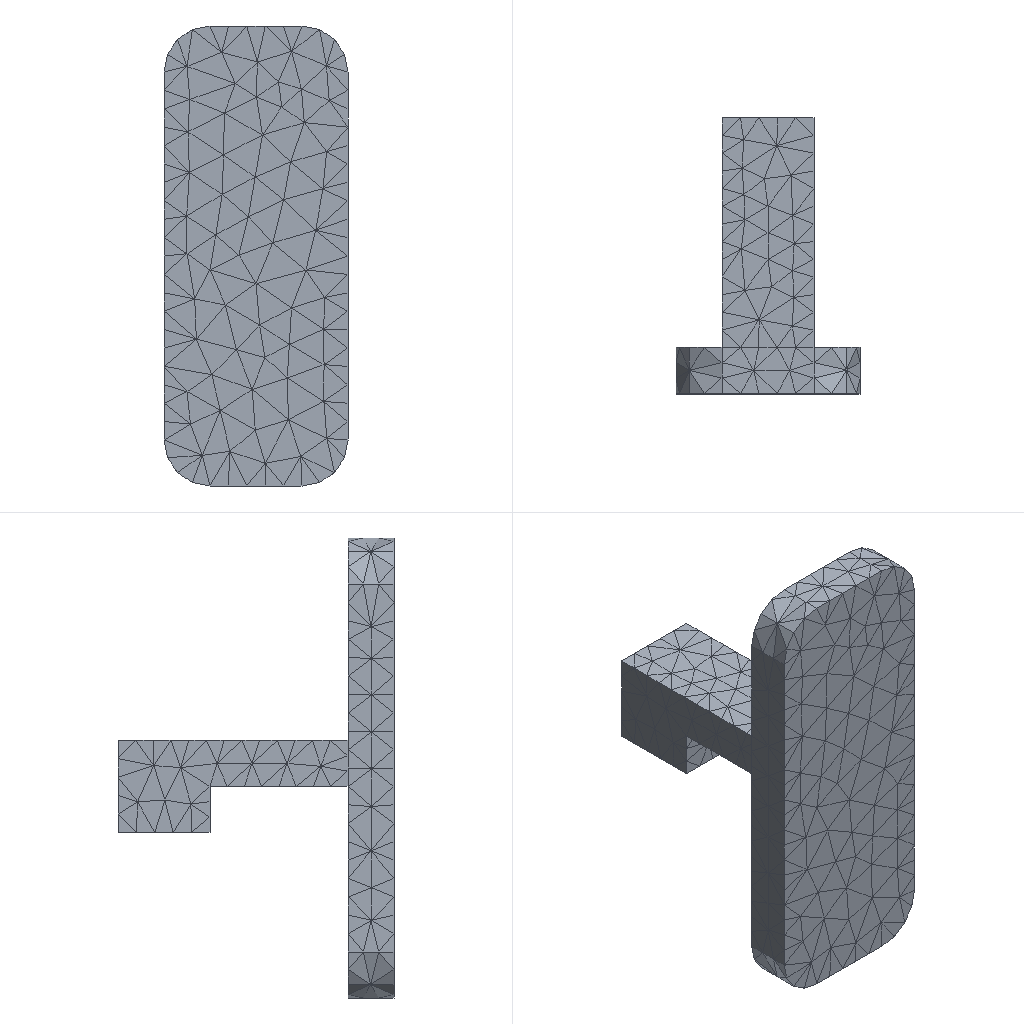Simulation study | ansys workbench
Ansys APDL input file, long lists of numbers shortened:
/batch
/config,noeldb,1     ! force off writing results to database
*get,_wallstrt,active,,time,wall
! ANSYS input file written by Workbench version 2021 R1
! File used for geometry attach:
/title,111111--____ (B5)
! ****** Begin Custom Load Command Snippet ******
/COM, ACT Extensions:
/COM,     LSDYNA, 2021.1
/COM,
! ****** End   Custom Load Command Snippet ******
*DIM,_wb_ProjectScratch_dir,string,248
_wb_ProjectScratch_dir(1) = ''
*DIM,_wb_SolverFiles_dir,string,248
_wb_SolverFiles_dir(1) = ''
*DIM,_wb_userfiles_dir,string,248
_wb_userfiles_dir(1) = ''
/com,--- Data in consistent NMM units. See Solving Units in the help system for more information.
/units,MPA
/nopr
/wb,file,start              !  signify a WB generated input file
/prep7
! Turn off shape checking because checks already performed inside WB mesher.
! See help system for more information.
SHPP,OFF,,NOWARN
/nolist
etcon,set             ! allow ANSYS to choose best KEYOP's for 180x elements, resets any applicable keyopt to MAPDL defaults
/com,*********** Nodes for the whole assembly ***********
nblock,3,,3264
(1i9,3e20.9e3)
        1     5.000000000E+00     3.000000000E+01    -2.200000000E+01
! (2967 more lines like these left out)
-1
/wb,elem,start            !  set before creation of elements
/com,*********** Elements for Body 1 "SYS-1\__" ***********
et,1,187
eblock,19,solid,,1472
(19i9)
        1        1        1        1        0        0        0        0       10        0        1      427      525      428      482     2716     2719     2712     2715
! (2943 more lines like these left out)
-1
/wb,elem,end               !  done creating elements
/com,*********** Send User Defined Coordinate System(s) ***********
csys,0
toffst,273.15,  ! Temperature offset from absolute zero
/com,*********** Set Reference Temperature ***********
tref,22.
/wb,mat,start              !  starting to send materials
/com,*********** Send Materials ***********
Temperature = 'TEMP' ! Temperature
MP,DENS,1,7.85e-09,	! tonne mm^-3
MP,ALPX,1,1.2e-05,	! C^-1
MP,C,1,434000000,	! mm^2 s^-2 C^-1
MP,KXX,1,60.5,	! tonne mm s^-3 C^-1
MP,RSVX,1,0.00017,	! ohm mm
MP,EX,1,200000,	! tonne s^-2 mm^-1
MP,NUXY,1,0.3,
MP,MURX,1,10000,
/wb,mat,end                !  done sending materials
!************************* Model Summary ********************
!SYS-1\__,	结构钢,	matid,	1
!************************* End Model Summary ********************
! get the diagonal of the bounding box. Needed later for other things
*get,_xmin,node,,mnloc,x
*get,_ymin,node,,mnloc,y
*get,_zmin,node,,mnloc,z
*get,_xmax,node,,mxloc,x
*get,_ymax,node,,mxloc,y
*get,_zmax,node,,mxloc,z
_ASMDIAG=(_xmax-_xmin)*(_xmax-_xmin)+(_ymax-_ymin)*(_ymax-_ymin)+(_zmax-_zmin)*(_zmax-_zmin)
_ASMDIAG=SQRT(_ASMDIAG)
/wb,contact,start          !  starting to send contact
/wb,contact,end            !  done creating contacts
/golist
/wb,load,start             !  starting to send loads
/com,*********** Fixed Supports ***********
CMBLOCK,_FIXEDSU,NODE,      431
(8i10)
       165       168       169       170       171       172       175       178
! (53 more lines like these left out)
cmsel,s,_FIXEDSU
d,all,all
nsel,all
/com,*********** Define Force Using Surface Effect Elements ***********
local,12,0,0.,0.,0.,0.,0.,0.
csys,0
et,2,154
eblock,10,,,28
(15i9)
     2367        2        2        2       12       72      429       73       73      886      889       73      883
! (27 more lines like these left out)
-1
esel,s,type,,2
keyop,2,2,1                ! Apply load in local coordinate system
keyop,2,7,1                ! Use original area so load is constant in large deformation
esel,all
/gst,on,on
fini
*get,_numnode,node,0,count
*get,_numelem,elem,0,count
*get, _MAXELEMNUM, elem, 0, NUM, MAX
*get, _MAXNODENUM, node, 0, NUM, MAX
*get, _MAXELEMTYPE, etyp, 0, NUM, MAX
*get, _MAXREALCONST, real, 0, NUM, MAX
/go
/wb,load,end               !  done creating loads
/com,--- Number of total nodes = %_numnode%
/com,--- Number of contact elements = 28
/com,--- Number of spring elements = 0
/com,--- Number of bearing elements = 0
/com,--- Number of solid elements = 1472
/com,--- Number of condensed parts = 0
/com,--- Number of total elements = %_numelem%
*get,_wallbsol,active,,time,wall
/com,****************************************************************************
/com,*************************    SOLUTION       ********************************
/com,****************************************************************************
/solu
antype,0                   ! static analysis
_thickRatio=  1     ! Ratio of thick parts in the model
eqsl,pcg,1e-8,,,,,,1
cntr,print,1               ! print out contact info and also make no initial contact an error
dmpoption,emat,no             ! Don't combine emat file for DANSYS
dmpoption,esav,no             ! Don't combine esav file for DANSYS
nldiag,cont,iter           ! print out contact info each equilibrium iteration
rescontrol,,none                 ! Do not keep any restart files
/com,****************************************************
/com,******************* SOLVE FOR LS 1 OF 1 ****************
esel,s,type,,2
nsle
sfe,all,1,pres,1,0.
sfe,all,2,pres,1,0.
sfe,all,3,pres,1,5.
nsel,all
esel,all
/nopr
/gopr
/nolist
nsub,1,1,1
time,1.
outres,erase
outres,all,none
outres,nsol,all,
outres,rsol,all
outres,eangl,all
outres,etmp,all
outres,veng,all
outres,strs,all,
outres,epel,all,
outres,eppl,all,
outres,cont,all,
! *********** WB SOLVE COMMAND ***********
! check interactive state
*get,ANSINTER_,active,,int
*if,ANSINTER_,ne,0,then
/eof
*endif
solve
/com *************** Write FE CONNECTORS *********
CEWRITE,file,ce,,INTE
/com,****************************************************
/com,*************** FINISHED SOLVE FOR LS 1 *************
*get,_wallasol,active,,time,wall
/nopr
*get,_numnode,node,0,count
*get,_numelem,elem,0,count
*get, _MAXELEMNUM, elem, 0, NUM, MAX
*get, _MAXNODENUM, node, 0, NUM, MAX,,,INTERNAL
*get, _MAXELEMTYPE, etyp, 0, NUM, MAX
*get, _MAXREALCONST, real, 0, NUM, MAX
/gopr
*get,_PCGITER,active,,solu,cgiter
/post1
xmlo,ENCODING,ISO-8859-1
xmlo,parm
/xml,parm,xml
fini
/gopr
*get,_walldone,active,,time,wall
_preptime=(_wallbsol-_wallstrt)*3600
_solvtime=(_wallasol-_wallbsol)*3600
_posttime=(_walldone-_wallasol)*3600
_totaltim=(_walldone-_wallstrt)*3600
*get,_dlbratio,active,0,solu,dlbr
*get,_combtime,active,0,solu,comb
/com,--- Total number of nodes = %_numnode%
/com,--- Total number of elements = %_numelem%
/com,--- Element load balance ratio = %_dlbratio%
/com,--- Time to combine distributed files = %_combtime%
/wb,file,end               ! done with WB generated input